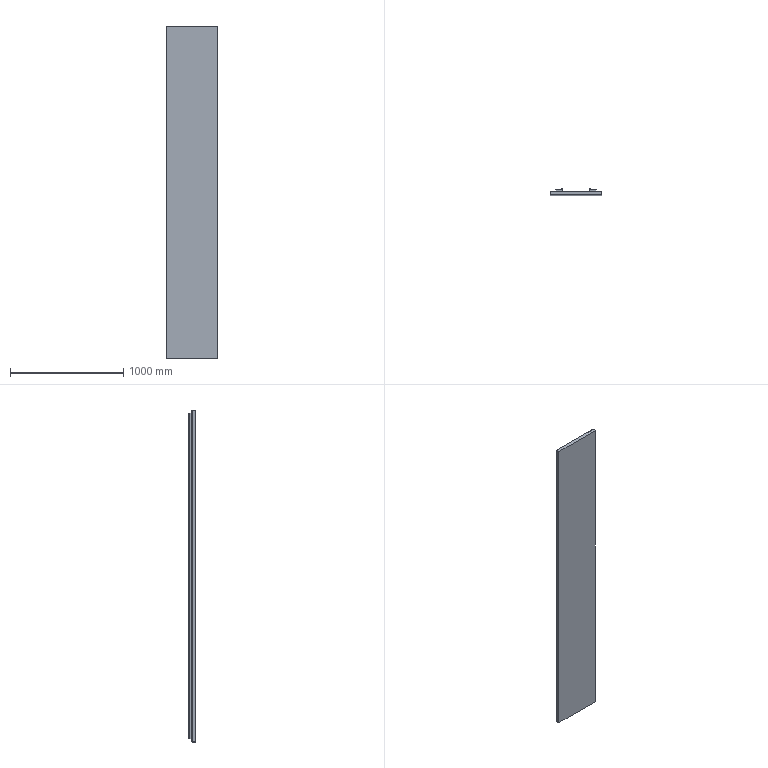Part | Creo | features DATUM PLANE 3, CHAMFER 2, CURVE 2, COORDINATE SYSTEM 1, CUT 1, PROTRUSION 1 | 1 solid | 36 faces | volume 47662635 mm3 | plane 36